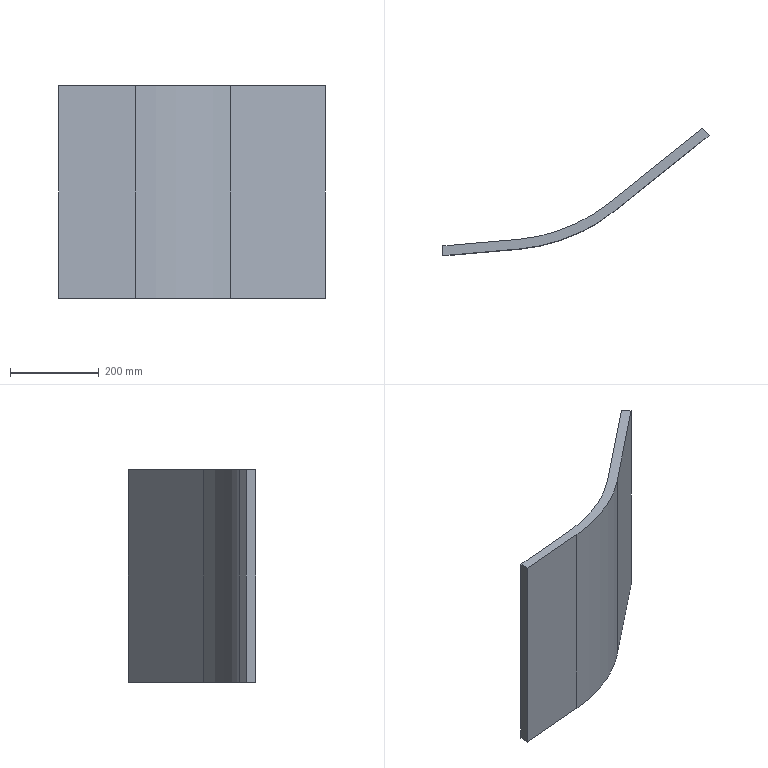Part | NX | features 底座(默认<按焊接>) 2 | 1 solid | 10 faces | box 600.05 x 287.774 x 480 mm | volume 7044002 mm3 | plane 8 | cylinder 2 | commonest cylinder face diameters 756.36 x1 800 x1
STEP:
#1=CARTESIAN_POINT('',(399.702,529.847,-412.));
#2=VERTEX_POINT('',#1);
#3=CARTESIAN_POINT('',(185.702,359.623,-412.));
#4=VERTEX_POINT('',#3);
#5=CARTESIAN_POINT('',(-493.475,-180.619,-412.));
#6=DIRECTION('',(-0.7826,-0.6225,0.));
#7=VECTOR('',#6,1000.);
#8=LINE('',#5,#7);
#9=EDGE_CURVE('',#2,#4,#8,.T.);
#10=ORIENTED_EDGE('',*,*,#9,.F.);
#11=CARTESIAN_POINT('',(399.702,529.847,-892.));
#12=VERTEX_POINT('',#11);
#13=CARTESIAN_POINT('',(399.702,529.847,-892.));
#14=DIRECTION('',(0.,0.,1.));
#15=VECTOR('',#14,1000.);
#16=LINE('',#13,#15);
#17=EDGE_CURVE('',#12,#2,#16,.T.);
#18=ORIENTED_EDGE('',*,*,#17,.F.);
#19=CARTESIAN_POINT('',(185.702,359.623,-892.));
#20=VERTEX_POINT('',#19);
#21=CARTESIAN_POINT('',(-493.475,-180.619,-892.));
#22=DIRECTION('',(-0.7826,-0.6225,0.));
#23=VECTOR('',#22,1000.);
#24=LINE('',#21,#23);
#25=EDGE_CURVE('',#12,#20,#24,.T.);
#26=ORIENTED_EDGE('',*,*,#25,.T.);
#27=CARTESIAN_POINT('',(185.702,359.623,-892.));
#28=DIRECTION('',(0.,0.,1.));
#29=VECTOR('',#28,1000.);
#30=LINE('',#27,#29);
#31=EDGE_CURVE('',#20,#4,#30,.T.);
#32=ORIENTED_EDGE('',*,*,#31,.T.);
#33=EDGE_LOOP('',(#10,#18,#26,#32));
#34=FACE_BOUND('',#33,.T.);
#35=CARTESIAN_POINT('',(-493.475,-180.619,-892.));
#36=DIRECTION('',(0.6225,-0.7826,0.));
#37=DIRECTION('',(0.7826,0.6225,0.));
#38=AXIS2_PLACEMENT_3D('',#35,#36,#37);
#39=PLANE('',#38);
#40=ADVANCED_FACE('',(#34),#39,.F.);
#41=CARTESIAN_POINT('',(-16.76,278.849,-412.));
#42=VERTEX_POINT('',#41);
#43=CARTESIAN_POINT('',(-49.72,655.59,-412.));
#44=DIRECTION('',(0.,0.,1.));
#45=DIRECTION('',(1.,0.,0.));
#46=AXIS2_PLACEMENT_3D('',#43,#44,#45);
#47=CIRCLE('',#46,378.18);
#48=EDGE_CURVE('',#4,#42,#47,.F.);
#49=ORIENTED_EDGE('',*,*,#48,.F.);
#50=ORIENTED_EDGE('',*,*,#31,.F.);
#51=CARTESIAN_POINT('',(-16.76,278.849,-892.));
#52=VERTEX_POINT('',#51);
#53=CARTESIAN_POINT('',(-49.72,655.59,-892.));
#54=DIRECTION('',(0.,0.,1.));
#55=DIRECTION('',(1.,0.,0.));
#56=AXIS2_PLACEMENT_3D('',#53,#54,#55);
#57=CIRCLE('',#56,378.18);
#58=EDGE_CURVE('',#20,#52,#57,.F.);
#59=ORIENTED_EDGE('',*,*,#58,.T.);
#60=CARTESIAN_POINT('',(-16.76,278.849,-892.));
#61=DIRECTION('',(0.,0.,1.));
#62=VECTOR('',#61,1000.);
#63=LINE('',#60,#62);
#64=EDGE_CURVE('',#52,#42,#63,.T.);
#65=ORIENTED_EDGE('',*,*,#64,.T.);
#66=EDGE_LOOP('',(#49,#50,#59,#65));
#67=FACE_BOUND('',#66,.T.);
#68=CARTESIAN_POINT('',(-49.72,655.59,-892.));
#69=DIRECTION('',(0.,0.,1.));
#70=DIRECTION('',(-1.,0.,0.));
#71=AXIS2_PLACEMENT_3D('',#68,#69,#70);
#72=CYLINDRICAL_SURFACE('',#71,378.18);
#73=ADVANCED_FACE('',(#67),#72,.F.);
#74=CARTESIAN_POINT('',(-186.765,263.976,-412.));
#75=VERTEX_POINT('',#74);
#76=CARTESIAN_POINT('',(1010.93,368.76,-412.));
#77=DIRECTION('',(-0.9962,-0.08716,0.));
#78=VECTOR('',#77,1000.);
#79=LINE('',#76,#78);
#80=EDGE_CURVE('',#42,#75,#79,.T.);
#81=ORIENTED_EDGE('',*,*,#80,.F.);
#82=ORIENTED_EDGE('',*,*,#64,.F.);
#83=CARTESIAN_POINT('',(-186.765,263.976,-892.));
#84=VERTEX_POINT('',#83);
#85=CARTESIAN_POINT('',(1010.93,368.76,-892.));
#86=DIRECTION('',(-0.9962,-0.08716,0.));
#87=VECTOR('',#86,1000.);
#88=LINE('',#85,#87);
#89=EDGE_CURVE('',#52,#84,#88,.T.);
#90=ORIENTED_EDGE('',*,*,#89,.T.);
#91=CARTESIAN_POINT('',(-186.765,263.976,-892.));
#92=DIRECTION('',(0.,0.,1.));
#93=VECTOR('',#92,1000.);
#94=LINE('',#91,#93);
#95=EDGE_CURVE('',#84,#75,#94,.T.);
#96=ORIENTED_EDGE('',*,*,#95,.T.);
#97=EDGE_LOOP('',(#81,#82,#90,#96));
#98=FACE_BOUND('',#97,.T.);
#99=CARTESIAN_POINT('',(1010.93,368.76,-892.));
#100=DIRECTION('',(0.08716,-0.9962,0.));
#101=DIRECTION('',(0.9962,0.08716,0.));
#102=AXIS2_PLACEMENT_3D('',#99,#100,#101);
#103=PLANE('',#102);
#104=ADVANCED_FACE('',(#98),#103,.F.);
#105=CARTESIAN_POINT('',(-186.765,242.072,-412.));
#106=VERTEX_POINT('',#105);
#107=CARTESIAN_POINT('',(-186.765,-2373.536,-412.));
#108=DIRECTION('',(0.,-1.,0.));
#109=VECTOR('',#108,1000.);
#110=LINE('',#107,#109);
#111=EDGE_CURVE('',#75,#106,#110,.T.);
#112=ORIENTED_EDGE('',*,*,#111,.F.);
#113=ORIENTED_EDGE('',*,*,#95,.F.);
#114=CARTESIAN_POINT('',(-186.765,242.072,-892.));
#115=VERTEX_POINT('',#114);
#116=CARTESIAN_POINT('',(-186.765,-2373.536,-892.));
#117=DIRECTION('',(0.,-1.,0.));
#118=VECTOR('',#117,1000.);
#119=LINE('',#116,#118);
#120=EDGE_CURVE('',#84,#115,#119,.T.);
#121=ORIENTED_EDGE('',*,*,#120,.T.);
#122=CARTESIAN_POINT('',(-186.765,242.072,-892.));
#123=DIRECTION('',(0.,0.,1.));
#124=VECTOR('',#123,1000.);
#125=LINE('',#122,#124);
#126=EDGE_CURVE('',#115,#106,#125,.T.);
#127=ORIENTED_EDGE('',*,*,#126,.T.);
#128=EDGE_LOOP('',(#112,#113,#121,#127));
#129=FACE_BOUND('',#128,.T.);
#130=CARTESIAN_POINT('',(-186.765,-2373.536,-892.));
#131=DIRECTION('',(1.,0.,0.));
#132=DIRECTION('',(0.,1.,0.));
#133=AXIS2_PLACEMENT_3D('',#130,#131,#132);
#134=PLANE('',#133);
#135=ADVANCED_FACE('',(#129),#134,.F.);
#136=CARTESIAN_POINT('',(-14.858,257.112,-412.));
#137=VERTEX_POINT('',#136);
#138=CARTESIAN_POINT('',(1012.832,347.024,-412.));
#139=DIRECTION('',(-0.9962,-0.08716,0.));
#140=VECTOR('',#139,1000.);
#141=LINE('',#138,#140);
#142=EDGE_CURVE('',#137,#106,#141,.T.);
#143=ORIENTED_EDGE('',*,*,#142,.T.);
#144=ORIENTED_EDGE('',*,*,#126,.F.);
#145=CARTESIAN_POINT('',(-14.858,257.112,-892.));
#146=VERTEX_POINT('',#145);
#147=CARTESIAN_POINT('',(1012.832,347.024,-892.));
#148=DIRECTION('',(-0.9962,-0.08716,0.));
#149=VECTOR('',#148,1000.);
#150=LINE('',#147,#149);
#151=EDGE_CURVE('',#146,#115,#150,.T.);
#152=ORIENTED_EDGE('',*,*,#151,.F.);
#153=CARTESIAN_POINT('',(-14.858,257.112,-892.));
#154=DIRECTION('',(0.,0.,1.));
#155=VECTOR('',#154,1000.);
#156=LINE('',#153,#155);
#157=EDGE_CURVE('',#146,#137,#156,.T.);
#158=ORIENTED_EDGE('',*,*,#157,.T.);
#159=EDGE_LOOP('',(#143,#144,#152,#158));
#160=FACE_BOUND('',#159,.T.);
#161=CARTESIAN_POINT('',(1012.832,347.024,-892.));
#162=DIRECTION('',(0.08716,-0.9962,0.));
#163=DIRECTION('',(0.9962,0.08716,0.));
#164=AXIS2_PLACEMENT_3D('',#161,#162,#163);
#165=PLANE('',#164);
#166=ADVANCED_FACE('',(#160),#165,.T.);
#167=CARTESIAN_POINT('',(199.285,342.547,-412.));
#168=VERTEX_POINT('',#167);
#169=CARTESIAN_POINT('',(-49.72,655.59,-412.));
#170=DIRECTION('',(0.,0.,1.));
#171=DIRECTION('',(1.,0.,0.));
#172=AXIS2_PLACEMENT_3D('',#169,#170,#171);
#173=CIRCLE('',#172,400.);
#174=EDGE_CURVE('',#168,#137,#173,.F.);
#175=ORIENTED_EDGE('',*,*,#174,.T.);
#176=ORIENTED_EDGE('',*,*,#157,.F.);
#177=CARTESIAN_POINT('',(199.285,342.547,-892.));
#178=VERTEX_POINT('',#177);
#179=CARTESIAN_POINT('',(-49.72,655.59,-892.));
#180=DIRECTION('',(0.,0.,1.));
#181=DIRECTION('',(1.,0.,0.));
#182=AXIS2_PLACEMENT_3D('',#179,#180,#181);
#183=CIRCLE('',#182,400.);
#184=EDGE_CURVE('',#178,#146,#183,.F.);
#185=ORIENTED_EDGE('',*,*,#184,.F.);
#186=CARTESIAN_POINT('',(199.285,342.547,-892.));
#187=DIRECTION('',(0.,0.,1.));
#188=VECTOR('',#187,1000.);
#189=LINE('',#186,#188);
#190=EDGE_CURVE('',#178,#168,#189,.T.);
#191=ORIENTED_EDGE('',*,*,#190,.T.);
#192=EDGE_LOOP('',(#175,#176,#185,#191));
#193=FACE_BOUND('',#192,.T.);
#194=CARTESIAN_POINT('',(-49.72,655.59,-892.));
#195=DIRECTION('',(0.,0.,1.));
#196=DIRECTION('',(-1.,0.,0.));
#197=AXIS2_PLACEMENT_3D('',#194,#195,#196);
#198=CYLINDRICAL_SURFACE('',#197,400.);
#199=ADVANCED_FACE('',(#193),#198,.T.);
#200=CARTESIAN_POINT('',(413.285,512.77,-412.));
#201=VERTEX_POINT('',#200);
#202=CARTESIAN_POINT('',(-479.892,-197.695,-412.));
#203=DIRECTION('',(-0.7826,-0.6225,0.));
#204=VECTOR('',#203,1000.);
#205=LINE('',#202,#204);
#206=EDGE_CURVE('',#201,#168,#205,.T.);
#207=ORIENTED_EDGE('',*,*,#206,.T.);
#208=ORIENTED_EDGE('',*,*,#190,.F.);
#209=CARTESIAN_POINT('',(413.285,512.77,-892.));
#210=VERTEX_POINT('',#209);
#211=CARTESIAN_POINT('',(-479.892,-197.695,-892.));
#212=DIRECTION('',(-0.7826,-0.6225,0.));
#213=VECTOR('',#212,1000.);
#214=LINE('',#211,#213);
#215=EDGE_CURVE('',#210,#178,#214,.T.);
#216=ORIENTED_EDGE('',*,*,#215,.F.);
#217=CARTESIAN_POINT('',(413.285,512.77,-892.));
#218=DIRECTION('',(0.,0.,1.));
#219=VECTOR('',#218,1000.);
#220=LINE('',#217,#219);
#221=EDGE_CURVE('',#210,#201,#220,.T.);
#222=ORIENTED_EDGE('',*,*,#221,.T.);
#223=EDGE_LOOP('',(#207,#208,#216,#222));
#224=FACE_BOUND('',#223,.T.);
#225=CARTESIAN_POINT('',(-479.892,-197.695,-892.));
#226=DIRECTION('',(0.6225,-0.7826,0.));
#227=DIRECTION('',(0.7826,0.6225,0.));
#228=AXIS2_PLACEMENT_3D('',#225,#226,#227);
#229=PLANE('',#228);
#230=ADVANCED_FACE('',(#224),#229,.T.);
#231=CARTESIAN_POINT('',(2144.027,-1663.071,-412.));
#232=DIRECTION('',(0.6225,-0.7826,0.));
#233=VECTOR('',#232,1000.);
#234=LINE('',#231,#233);
#235=EDGE_CURVE('',#2,#201,#234,.T.);
#236=ORIENTED_EDGE('',*,*,#235,.T.);
#237=ORIENTED_EDGE('',*,*,#221,.F.);
#238=CARTESIAN_POINT('',(2144.027,-1663.071,-892.));
#239=DIRECTION('',(0.6225,-0.7826,0.));
#240=VECTOR('',#239,1000.);
#241=LINE('',#238,#240);
#242=EDGE_CURVE('',#12,#210,#241,.T.);
#243=ORIENTED_EDGE('',*,*,#242,.F.);
#244=ORIENTED_EDGE('',*,*,#17,.T.);
#245=EDGE_LOOP('',(#236,#237,#243,#244));
#246=FACE_BOUND('',#245,.T.);
#247=CARTESIAN_POINT('',(2144.027,-1663.071,-892.));
#248=DIRECTION('',(0.7826,0.6225,0.));
#249=DIRECTION('',(-0.6225,0.7826,0.));
#250=AXIS2_PLACEMENT_3D('',#247,#248,#249);
#251=PLANE('',#250);
#252=ADVANCED_FACE('',(#246),#251,.T.);
#253=ORIENTED_EDGE('',*,*,#25,.F.);
#254=ORIENTED_EDGE('',*,*,#242,.T.);
#255=ORIENTED_EDGE('',*,*,#215,.T.);
#256=ORIENTED_EDGE('',*,*,#184,.T.);
#257=ORIENTED_EDGE('',*,*,#151,.T.);
#258=ORIENTED_EDGE('',*,*,#120,.F.);
#259=ORIENTED_EDGE('',*,*,#89,.F.);
#260=ORIENTED_EDGE('',*,*,#58,.F.);
#261=EDGE_LOOP('',(#253,#254,#255,#256,#257,#258,#259,#260));
#262=FACE_BOUND('',#261,.T.);
#263=CARTESIAN_POINT('',(1250.85,-2373.536,-892.));
#264=DIRECTION('',(0.,0.,-1.));
#265=DIRECTION('',(1.,0.,0.));
#266=AXIS2_PLACEMENT_3D('',#263,#264,#265);
#267=PLANE('',#266);
#268=ADVANCED_FACE('',(#262),#267,.T.);
#269=ORIENTED_EDGE('',*,*,#9,.T.);
#270=ORIENTED_EDGE('',*,*,#48,.T.);
#271=ORIENTED_EDGE('',*,*,#80,.T.);
#272=ORIENTED_EDGE('',*,*,#111,.T.);
#273=ORIENTED_EDGE('',*,*,#142,.F.);
#274=ORIENTED_EDGE('',*,*,#174,.F.);
#275=ORIENTED_EDGE('',*,*,#206,.F.);
#276=ORIENTED_EDGE('',*,*,#235,.F.);
#277=EDGE_LOOP('',(#269,#270,#271,#272,#273,#274,#275,#276));
#278=FACE_BOUND('',#277,.T.);
#279=CARTESIAN_POINT('',(1250.85,-2373.536,-412.));
#280=DIRECTION('',(0.,0.,-1.));
#281=DIRECTION('',(1.,0.,0.));
#282=AXIS2_PLACEMENT_3D('',#279,#280,#281);
#283=PLANE('',#282);
#284=ADVANCED_FACE('',(#278),#283,.F.);
#285=CLOSED_SHELL('',(#40,#73,#104,#135,#166,#199,#230,#252,#268,#284));
#286=MANIFOLD_SOLID_BREP('',#285);
#287=(LENGTH_UNIT()NAMED_UNIT(*)SI_UNIT(.MILLI.,.METRE.));
#288=UNCERTAINTY_MEASURE_WITH_UNIT(LENGTH_MEASURE(0.00001),#287,'','');
#289=(NAMED_UNIT(*)PLANE_ANGLE_UNIT()SI_UNIT($,.RADIAN.));
#290=(NAMED_UNIT(*)SI_UNIT($,.STERADIAN.)SOLID_ANGLE_UNIT());
#291=(GEOMETRIC_REPRESENTATION_CONTEXT(3)GLOBAL_UNCERTAINTY_ASSIGNED_CONTEXT((#288))GLOBAL_UNIT_ASSIGNED_CONTEXT((#287,#289,#290))REPRESENTATION_CONTEXT('',''));
#292=ADVANCED_BREP_SHAPE_REPRESENTATION('',(#286),#291);